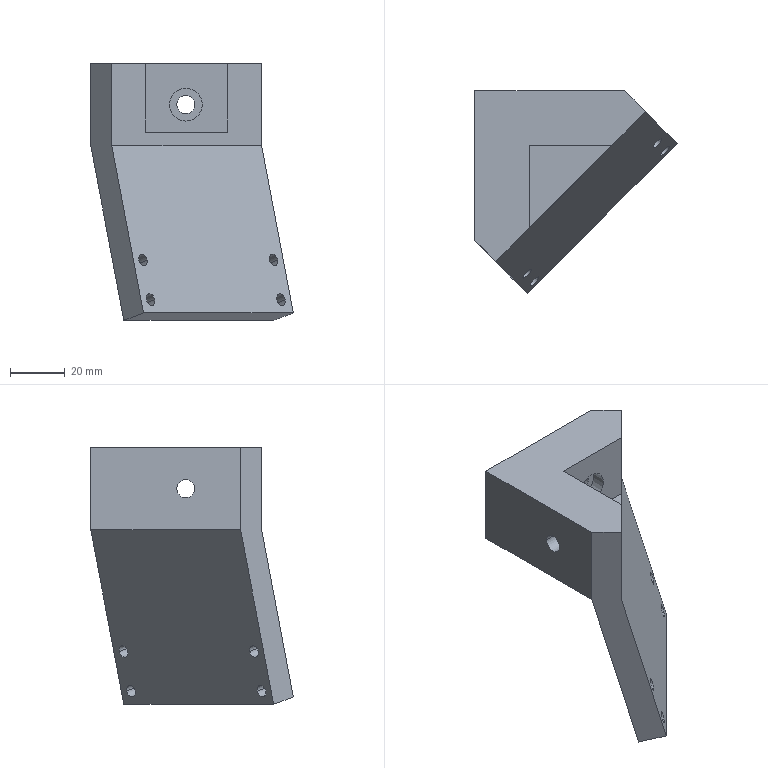Part | SolidWorks | features ICE 6, Extrusion 1, MirrorPattern 1 | 1 solid | 31 faces | box 73.918 x 73.918 x 93.747 mm | volume 108156 mm3 | cylinder 16 | plane 15 | commonest cylinder face diameters 4.4 x8 6.6 x4 12 x4
STEP:
#1=CARTESIAN_POINT('',(10.398,-61.143,-59.429));
#2=VERTEX_POINT('',#1);
#3=CARTESIAN_POINT('',(13.509,-58.031,-59.429));
#4=VERTEX_POINT('',#3);
#5=CARTESIAN_POINT('',(11.953,-59.587,-59.429));
#6=DIRECTION('',(0.683,-0.683,0.2588));
#7=DIRECTION('',(0.7071,0.7071,0.));
#8=AXIS2_PLACEMENT_3D('',#5,#6,#7);
#9=CIRCLE('',#8,2.2);
#10=EDGE_CURVE('',#2,#4,#9,.T.);
#11=ORIENTED_EDGE('',*,*,#10,.F.);
#12=CARTESIAN_POINT('',(17.533,-68.278,-56.725));
#13=VERTEX_POINT('',#12);
#14=CARTESIAN_POINT('',(-2.957,-47.788,-64.49));
#15=DIRECTION('',(0.683,-0.683,0.2588));
#16=VECTOR('',#15,1000.);
#17=LINE('',#14,#16);
#18=EDGE_CURVE('',#2,#13,#17,.T.);
#19=ORIENTED_EDGE('',*,*,#18,.T.);
#20=CARTESIAN_POINT('',(20.644,-65.167,-56.725));
#21=VERTEX_POINT('',#20);
#22=CARTESIAN_POINT('',(19.089,-66.722,-56.725));
#23=DIRECTION('',(0.683,-0.683,0.2588));
#24=DIRECTION('',(0.7071,0.7071,0.));
#25=AXIS2_PLACEMENT_3D('',#22,#23,#24);
#26=CIRCLE('',#25,2.2);
#27=EDGE_CURVE('',#13,#21,#26,.T.);
#28=ORIENTED_EDGE('',*,*,#27,.T.);
#29=CARTESIAN_POINT('',(0.1541,-44.676,-64.49));
#30=DIRECTION('',(0.683,-0.683,0.2588));
#31=VECTOR('',#30,1000.);
#32=LINE('',#29,#31);
#33=EDGE_CURVE('',#4,#21,#32,.T.);
#34=ORIENTED_EDGE('',*,*,#33,.F.);
#35=EDGE_LOOP('',(#11,#19,#28,#34));
#36=FACE_OUTER_BOUND('',#35,.T.);
#37=CARTESIAN_POINT('',(-1.402,-46.232,-64.49));
#38=DIRECTION('',(0.683,-0.683,0.2588));
#39=DIRECTION('',(0.7071,0.7071,0.));
#40=AXIS2_PLACEMENT_3D('',#37,#38,#39);
#41=CYLINDRICAL_SURFACE('',#40,2.2);
#42=ADVANCED_FACE('',(#36),#41,.F.);
#43=CARTESIAN_POINT('',(13.143,-63.888,-73.918));
#44=VERTEX_POINT('',#43);
#45=CARTESIAN_POINT('',(16.254,-60.776,-73.918));
#46=VERTEX_POINT('',#45);
#47=CARTESIAN_POINT('',(14.699,-62.332,-73.918));
#48=DIRECTION('',(0.683,-0.683,0.2588));
#49=DIRECTION('',(0.7071,0.7071,0.));
#50=AXIS2_PLACEMENT_3D('',#47,#48,#49);
#51=CIRCLE('',#50,2.2);
#52=EDGE_CURVE('',#44,#46,#51,.T.);
#53=ORIENTED_EDGE('',*,*,#52,.F.);
#54=CARTESIAN_POINT('',(20.278,-71.023,-71.214));
#55=VERTEX_POINT('',#54);
#56=CARTESIAN_POINT('',(-0.212,-50.533,-78.978));
#57=DIRECTION('',(0.683,-0.683,0.2588));
#58=VECTOR('',#57,1000.);
#59=LINE('',#56,#58);
#60=EDGE_CURVE('',#44,#55,#59,.T.);
#61=ORIENTED_EDGE('',*,*,#60,.T.);
#62=CARTESIAN_POINT('',(23.39,-67.912,-71.214));
#63=VERTEX_POINT('',#62);
#64=CARTESIAN_POINT('',(21.834,-69.468,-71.214));
#65=DIRECTION('',(0.683,-0.683,0.2588));
#66=DIRECTION('',(0.7071,0.7071,0.));
#67=AXIS2_PLACEMENT_3D('',#64,#65,#66);
#68=CIRCLE('',#67,2.2);
#69=EDGE_CURVE('',#55,#63,#68,.T.);
#70=ORIENTED_EDGE('',*,*,#69,.T.);
#71=CARTESIAN_POINT('',(2.899,-47.422,-78.978));
#72=DIRECTION('',(0.683,-0.683,0.2588));
#73=VECTOR('',#72,1000.);
#74=LINE('',#71,#73);
#75=EDGE_CURVE('',#46,#63,#74,.T.);
#76=ORIENTED_EDGE('',*,*,#75,.F.);
#77=EDGE_LOOP('',(#53,#61,#70,#76));
#78=FACE_OUTER_BOUND('',#77,.T.);
#79=CARTESIAN_POINT('',(1.344,-48.977,-78.978));
#80=DIRECTION('',(0.683,-0.683,0.2588));
#81=DIRECTION('',(0.7071,0.7071,0.));
#82=AXIS2_PLACEMENT_3D('',#79,#80,#81);
#83=CYLINDRICAL_SURFACE('',#82,2.2);
#84=ADVANCED_FACE('',(#78),#83,.F.);
#85=CARTESIAN_POINT('',(60.776,-16.254,-73.918));
#86=VERTEX_POINT('',#85);
#87=CARTESIAN_POINT('',(63.888,-13.143,-73.918));
#88=VERTEX_POINT('',#87);
#89=CARTESIAN_POINT('',(62.332,-14.699,-73.918));
#90=DIRECTION('',(0.683,-0.683,0.2588));
#91=DIRECTION('',(0.7071,0.7071,0.));
#92=AXIS2_PLACEMENT_3D('',#89,#90,#91);
#93=CIRCLE('',#92,2.2);
#94=EDGE_CURVE('',#86,#88,#93,.T.);
#95=ORIENTED_EDGE('',*,*,#94,.F.);
#96=CARTESIAN_POINT('',(67.912,-23.39,-71.214));
#97=VERTEX_POINT('',#96);
#98=CARTESIAN_POINT('',(47.422,-2.899,-78.978));
#99=DIRECTION('',(0.683,-0.683,0.2588));
#100=VECTOR('',#99,1000.);
#101=LINE('',#98,#100);
#102=EDGE_CURVE('',#86,#97,#101,.T.);
#103=ORIENTED_EDGE('',*,*,#102,.T.);
#104=CARTESIAN_POINT('',(71.023,-20.278,-71.214));
#105=VERTEX_POINT('',#104);
#106=CARTESIAN_POINT('',(69.468,-21.834,-71.214));
#107=DIRECTION('',(0.683,-0.683,0.2588));
#108=DIRECTION('',(0.7071,0.7071,0.));
#109=AXIS2_PLACEMENT_3D('',#106,#107,#108);
#110=CIRCLE('',#109,2.2);
#111=EDGE_CURVE('',#97,#105,#110,.T.);
#112=ORIENTED_EDGE('',*,*,#111,.T.);
#113=CARTESIAN_POINT('',(50.533,0.212,-78.978));
#114=DIRECTION('',(0.683,-0.683,0.2588));
#115=VECTOR('',#114,1000.);
#116=LINE('',#113,#115);
#117=EDGE_CURVE('',#88,#105,#116,.T.);
#118=ORIENTED_EDGE('',*,*,#117,.F.);
#119=EDGE_LOOP('',(#95,#103,#112,#118));
#120=FACE_OUTER_BOUND('',#119,.T.);
#121=CARTESIAN_POINT('',(48.977,-1.344,-78.978));
#122=DIRECTION('',(0.683,-0.683,0.2588));
#123=DIRECTION('',(0.7071,0.7071,0.));
#124=AXIS2_PLACEMENT_3D('',#121,#122,#123);
#125=CYLINDRICAL_SURFACE('',#124,2.2);
#126=ADVANCED_FACE('',(#120),#125,.F.);
#127=CARTESIAN_POINT('',(58.031,-13.509,-59.429));
#128=VERTEX_POINT('',#127);
#129=CARTESIAN_POINT('',(61.143,-10.398,-59.429));
#130=VERTEX_POINT('',#129);
#131=CARTESIAN_POINT('',(59.587,-11.953,-59.429));
#132=DIRECTION('',(0.683,-0.683,0.2588));
#133=DIRECTION('',(0.7071,0.7071,0.));
#134=AXIS2_PLACEMENT_3D('',#131,#132,#133);
#135=CIRCLE('',#134,2.2);
#136=EDGE_CURVE('',#128,#130,#135,.T.);
#137=ORIENTED_EDGE('',*,*,#136,.F.);
#138=CARTESIAN_POINT('',(65.167,-20.644,-56.725));
#139=VERTEX_POINT('',#138);
#140=CARTESIAN_POINT('',(44.676,-0.1541,-64.49));
#141=DIRECTION('',(0.683,-0.683,0.2588));
#142=VECTOR('',#141,1000.);
#143=LINE('',#140,#142);
#144=EDGE_CURVE('',#128,#139,#143,.T.);
#145=ORIENTED_EDGE('',*,*,#144,.T.);
#146=CARTESIAN_POINT('',(68.278,-17.533,-56.725));
#147=VERTEX_POINT('',#146);
#148=CARTESIAN_POINT('',(66.722,-19.089,-56.725));
#149=DIRECTION('',(0.683,-0.683,0.2588));
#150=DIRECTION('',(0.7071,0.7071,0.));
#151=AXIS2_PLACEMENT_3D('',#148,#149,#150);
#152=CIRCLE('',#151,2.2);
#153=EDGE_CURVE('',#139,#147,#152,.T.);
#154=ORIENTED_EDGE('',*,*,#153,.T.);
#155=CARTESIAN_POINT('',(47.788,2.957,-64.49));
#156=DIRECTION('',(0.683,-0.683,0.2588));
#157=VECTOR('',#156,1000.);
#158=LINE('',#155,#157);
#159=EDGE_CURVE('',#130,#147,#158,.T.);
#160=ORIENTED_EDGE('',*,*,#159,.F.);
#161=EDGE_LOOP('',(#137,#145,#154,#160));
#162=FACE_OUTER_BOUND('',#161,.T.);
#163=CARTESIAN_POINT('',(46.232,1.402,-64.49));
#164=DIRECTION('',(0.683,-0.683,0.2588));
#165=DIRECTION('',(0.7071,0.7071,0.));
#166=AXIS2_PLACEMENT_3D('',#163,#164,#165);
#167=CYLINDRICAL_SURFACE('',#166,2.2);
#168=ADVANCED_FACE('',(#162),#167,.F.);
#169=CARTESIAN_POINT('',(20.,-40.705,0.));
#170=VERTEX_POINT('',#169);
#171=CARTESIAN_POINT('',(20.,-28.705,0.));
#172=VERTEX_POINT('',#171);
#173=CARTESIAN_POINT('',(20.,-34.705,0.));
#174=DIRECTION('',(1.,0.,0.));
#175=DIRECTION('',(0.,-1.,0.));
#176=AXIS2_PLACEMENT_3D('',#173,#174,#175);
#177=CIRCLE('',#176,6.);
#178=EDGE_CURVE('',#170,#172,#177,.T.);
#179=ORIENTED_EDGE('',*,*,#178,.T.);
#180=CARTESIAN_POINT('',(15.,-28.705,0.));
#181=VERTEX_POINT('',#180);
#182=CARTESIAN_POINT('',(128.,-28.705,0.));
#183=DIRECTION('',(-1.,0.,0.));
#184=VECTOR('',#183,1000.);
#185=LINE('',#182,#184);
#186=EDGE_CURVE('',#172,#181,#185,.T.);
#187=ORIENTED_EDGE('',*,*,#186,.T.);
#188=CARTESIAN_POINT('',(15.,-40.705,0.));
#189=VERTEX_POINT('',#188);
#190=CARTESIAN_POINT('',(15.,-34.705,0.));
#191=DIRECTION('',(1.,0.,0.));
#192=DIRECTION('',(0.,0.,1.));
#193=AXIS2_PLACEMENT_3D('',#190,#191,#192);
#194=CIRCLE('',#193,6.);
#195=EDGE_CURVE('',#189,#181,#194,.T.);
#196=ORIENTED_EDGE('',*,*,#195,.F.);
#197=CARTESIAN_POINT('',(128.,-40.705,0.));
#198=DIRECTION('',(-1.,0.,0.));
#199=VECTOR('',#198,1000.);
#200=LINE('',#197,#199);
#201=EDGE_CURVE('',#170,#189,#200,.T.);
#202=ORIENTED_EDGE('',*,*,#201,.F.);
#203=EDGE_LOOP('',(#179,#187,#196,#202));
#204=FACE_OUTER_BOUND('',#203,.T.);
#205=CARTESIAN_POINT('',(128.,-34.705,0.));
#206=DIRECTION('',(-1.,0.,0.));
#207=DIRECTION('',(0.,-1.,0.));
#208=AXIS2_PLACEMENT_3D('',#205,#206,#207);
#209=CYLINDRICAL_SURFACE('',#208,6.);
#210=ADVANCED_FACE('',(#204),#209,.F.);
#211=CARTESIAN_POINT('',(15.,-31.405,0.));
#212=VERTEX_POINT('',#211);
#213=CARTESIAN_POINT('',(15.,-38.005,0.));
#214=VERTEX_POINT('',#213);
#215=CARTESIAN_POINT('',(15.,-34.705,0.));
#216=DIRECTION('',(-1.,0.,0.));
#217=DIRECTION('',(0.,-1.,0.));
#218=AXIS2_PLACEMENT_3D('',#215,#216,#217);
#219=CIRCLE('',#218,3.3);
#220=EDGE_CURVE('',#212,#214,#219,.T.);
#221=ORIENTED_EDGE('',*,*,#220,.F.);
#222=CARTESIAN_POINT('',(0.,-31.405,0.));
#223=VERTEX_POINT('',#222);
#224=CARTESIAN_POINT('',(113.,-31.405,0.));
#225=DIRECTION('',(-1.,0.,0.));
#226=VECTOR('',#225,1000.);
#227=LINE('',#224,#226);
#228=EDGE_CURVE('',#212,#223,#227,.T.);
#229=ORIENTED_EDGE('',*,*,#228,.T.);
#230=CARTESIAN_POINT('',(0.,-38.005,0.));
#231=VERTEX_POINT('',#230);
#232=CARTESIAN_POINT('',(0.,-34.705,0.));
#233=DIRECTION('',(1.,0.,0.));
#234=DIRECTION('',(0.,0.,1.));
#235=AXIS2_PLACEMENT_3D('',#232,#233,#234);
#236=CIRCLE('',#235,3.3);
#237=EDGE_CURVE('',#231,#223,#236,.T.);
#238=ORIENTED_EDGE('',*,*,#237,.F.);
#239=CARTESIAN_POINT('',(113.,-38.005,0.));
#240=DIRECTION('',(-1.,0.,0.));
#241=VECTOR('',#240,1000.);
#242=LINE('',#239,#241);
#243=EDGE_CURVE('',#214,#231,#242,.T.);
#244=ORIENTED_EDGE('',*,*,#243,.F.);
#245=EDGE_LOOP('',(#221,#229,#238,#244));
#246=FACE_OUTER_BOUND('',#245,.T.);
#247=CARTESIAN_POINT('',(113.,-34.705,0.));
#248=DIRECTION('',(-1.,0.,0.));
#249=DIRECTION('',(0.,-1.,0.));
#250=AXIS2_PLACEMENT_3D('',#247,#248,#249);
#251=CYLINDRICAL_SURFACE('',#250,3.3);
#252=ADVANCED_FACE('',(#246),#251,.F.);
#253=CARTESIAN_POINT('',(34.705,-20.,6.));
#254=VERTEX_POINT('',#253);
#255=CARTESIAN_POINT('',(34.705,-20.,-6.));
#256=VERTEX_POINT('',#255);
#257=CARTESIAN_POINT('',(34.705,-20.,0.));
#258=DIRECTION('',(0.,-1.,0.));
#259=DIRECTION('',(0.,0.,1.));
#260=AXIS2_PLACEMENT_3D('',#257,#258,#259);
#261=CIRCLE('',#260,6.);
#262=EDGE_CURVE('',#254,#256,#261,.T.);
#263=ORIENTED_EDGE('',*,*,#262,.T.);
#264=CARTESIAN_POINT('',(34.705,-15.,-6.));
#265=VERTEX_POINT('',#264);
#266=CARTESIAN_POINT('',(34.705,-128.,-6.));
#267=DIRECTION('',(0.,1.,0.));
#268=VECTOR('',#267,1000.);
#269=LINE('',#266,#268);
#270=EDGE_CURVE('',#256,#265,#269,.T.);
#271=ORIENTED_EDGE('',*,*,#270,.T.);
#272=CARTESIAN_POINT('',(34.705,-15.,6.));
#273=VERTEX_POINT('',#272);
#274=CARTESIAN_POINT('',(34.705,-15.,0.));
#275=DIRECTION('',(0.,1.,0.));
#276=DIRECTION('',(0.,0.,1.));
#277=AXIS2_PLACEMENT_3D('',#274,#275,#276);
#278=CIRCLE('',#277,6.);
#279=EDGE_CURVE('',#265,#273,#278,.T.);
#280=ORIENTED_EDGE('',*,*,#279,.T.);
#281=CARTESIAN_POINT('',(34.705,-128.,6.));
#282=DIRECTION('',(0.,1.,0.));
#283=VECTOR('',#282,1000.);
#284=LINE('',#281,#283);
#285=EDGE_CURVE('',#254,#273,#284,.T.);
#286=ORIENTED_EDGE('',*,*,#285,.F.);
#287=EDGE_LOOP('',(#263,#271,#280,#286));
#288=FACE_OUTER_BOUND('',#287,.T.);
#289=CARTESIAN_POINT('',(34.705,-128.,0.));
#290=DIRECTION('',(0.,1.,0.));
#291=DIRECTION('',(0.,0.,1.));
#292=AXIS2_PLACEMENT_3D('',#289,#290,#291);
#293=CYLINDRICAL_SURFACE('',#292,6.);
#294=ADVANCED_FACE('',(#288),#293,.F.);
#295=CARTESIAN_POINT('',(34.705,-15.,3.3));
#296=VERTEX_POINT('',#295);
#297=CARTESIAN_POINT('',(34.705,-15.,-3.3));
#298=VERTEX_POINT('',#297);
#299=CARTESIAN_POINT('',(34.705,-15.,0.));
#300=DIRECTION('',(0.,-1.,0.));
#301=DIRECTION('',(0.,0.,1.));
#302=AXIS2_PLACEMENT_3D('',#299,#300,#301);
#303=CIRCLE('',#302,3.3);
#304=EDGE_CURVE('',#296,#298,#303,.T.);
#305=ORIENTED_EDGE('',*,*,#304,.T.);
#306=CARTESIAN_POINT('',(34.705,0.,-3.3));
#307=VERTEX_POINT('',#306);
#308=CARTESIAN_POINT('',(34.705,-113.,-3.3));
#309=DIRECTION('',(0.,1.,0.));
#310=VECTOR('',#309,1000.);
#311=LINE('',#308,#310);
#312=EDGE_CURVE('',#298,#307,#311,.T.);
#313=ORIENTED_EDGE('',*,*,#312,.T.);
#314=CARTESIAN_POINT('',(34.705,0.,3.3));
#315=VERTEX_POINT('',#314);
#316=CARTESIAN_POINT('',(34.705,0.,0.));
#317=DIRECTION('',(0.,1.,0.));
#318=DIRECTION('',(0.,0.,1.));
#319=AXIS2_PLACEMENT_3D('',#316,#317,#318);
#320=CIRCLE('',#319,3.3);
#321=EDGE_CURVE('',#307,#315,#320,.T.);
#322=ORIENTED_EDGE('',*,*,#321,.T.);
#323=CARTESIAN_POINT('',(34.705,-113.,3.3));
#324=DIRECTION('',(0.,1.,0.));
#325=VECTOR('',#324,1000.);
#326=LINE('',#323,#325);
#327=EDGE_CURVE('',#296,#315,#326,.T.);
#328=ORIENTED_EDGE('',*,*,#327,.F.);
#329=EDGE_LOOP('',(#305,#313,#322,#328));
#330=FACE_OUTER_BOUND('',#329,.T.);
#331=CARTESIAN_POINT('',(34.705,-113.,0.));
#332=DIRECTION('',(0.,1.,0.));
#333=DIRECTION('',(0.,0.,1.));
#334=AXIS2_PLACEMENT_3D('',#331,#332,#333);
#335=CYLINDRICAL_SURFACE('',#334,3.3);
#336=ADVANCED_FACE('',(#330),#335,.F.);
#337=CARTESIAN_POINT('',(20.,-50.,-10.));
#338=VERTEX_POINT('',#337);
#339=CARTESIAN_POINT('',(50.,-20.,-10.));
#340=VERTEX_POINT('',#339);
#341=CARTESIAN_POINT('',(35.,-35.,-10.));
#342=DIRECTION('',(0.7071,0.7071,0.));
#343=VECTOR('',#342,1000.);
#344=LINE('',#341,#343);
#345=EDGE_CURVE('',#338,#340,#344,.T.);
#346=ORIENTED_EDGE('',*,*,#345,.F.);
#347=CARTESIAN_POINT('',(20.,-50.,15.));
#348=VERTEX_POINT('',#347);
#349=CARTESIAN_POINT('',(20.,-50.,-10.));
#350=DIRECTION('',(0.,0.,1.));
#351=VECTOR('',#350,1000.);
#352=LINE('',#349,#351);
#353=EDGE_CURVE('',#338,#348,#352,.T.);
#354=ORIENTED_EDGE('',*,*,#353,.T.);
#355=CARTESIAN_POINT('',(7.648,-62.352,15.));
#356=VERTEX_POINT('',#355);
#357=CARTESIAN_POINT('',(70.,0.,15.));
#358=DIRECTION('',(0.7071,0.7071,0.));
#359=VECTOR('',#358,1000.);
#360=LINE('',#357,#359);
#361=EDGE_CURVE('',#356,#348,#360,.T.);
#362=ORIENTED_EDGE('',*,*,#361,.F.);
#363=CARTESIAN_POINT('',(7.648,-62.352,-15.));
#364=VERTEX_POINT('',#363);
#365=CARTESIAN_POINT('',(7.648,-62.352,15.));
#366=DIRECTION('',(0.,0.,1.));
#367=VECTOR('',#366,1000.);
#368=LINE('',#365,#367);
#369=EDGE_CURVE('',#364,#356,#368,.T.);
#370=ORIENTED_EDGE('',*,*,#369,.F.);
#371=CARTESIAN_POINT('',(62.352,-7.648,-15.));
#372=VERTEX_POINT('',#371);
#373=CARTESIAN_POINT('',(70.,0.,-15.));
#374=DIRECTION('',(0.7071,0.7071,0.));
#375=VECTOR('',#374,1000.);
#376=LINE('',#373,#375);
#377=EDGE_CURVE('',#364,#372,#376,.T.);
#378=ORIENTED_EDGE('',*,*,#377,.T.);
#379=CARTESIAN_POINT('',(62.352,-7.648,15.));
#380=VERTEX_POINT('',#379);
#381=CARTESIAN_POINT('',(62.352,-7.648,15.));
#382=DIRECTION('',(0.,0.,1.));
#383=VECTOR('',#382,1000.);
#384=LINE('',#381,#383);
#385=EDGE_CURVE('',#372,#380,#384,.T.);
#386=ORIENTED_EDGE('',*,*,#385,.T.);
#387=CARTESIAN_POINT('',(50.,-20.,15.));
#388=VERTEX_POINT('',#387);
#389=CARTESIAN_POINT('',(70.,0.,15.));
#390=DIRECTION('',(0.7071,0.7071,0.));
#391=VECTOR('',#390,1000.);
#392=LINE('',#389,#391);
#393=EDGE_CURVE('',#388,#380,#392,.T.);
#394=ORIENTED_EDGE('',*,*,#393,.F.);
#395=CARTESIAN_POINT('',(50.,-20.,-10.));
#396=DIRECTION('',(0.,0.,1.));
#397=VECTOR('',#396,1000.);
#398=LINE('',#395,#397);
#399=EDGE_CURVE('',#340,#388,#398,.T.);
#400=ORIENTED_EDGE('',*,*,#399,.F.);
#401=EDGE_LOOP('',(#346,#354,#362,#370,#378,#386,#394,#400));
#402=FACE_OUTER_BOUND('',#401,.T.);
#403=CARTESIAN_POINT('',(70.,0.,15.));
#404=DIRECTION('',(-0.7071,0.7071,0.));
#405=DIRECTION('',(-0.7071,-0.7071,0.));
#406=AXIS2_PLACEMENT_3D('',#403,#404,#405);
#407=PLANE('',#406);
#408=ADVANCED_FACE('',(#402),#407,.F.);
#409=ORIENTED_EDGE('',*,*,#361,.T.);
#410=CARTESIAN_POINT('',(20.,-20.,15.));
#411=VERTEX_POINT('',#410);
#412=CARTESIAN_POINT('',(20.,0.,15.));
#413=DIRECTION('',(0.,-1.,0.));
#414=VECTOR('',#413,1000.);
#415=LINE('',#412,#414);
#416=EDGE_CURVE('',#411,#348,#415,.T.);
#417=ORIENTED_EDGE('',*,*,#416,.F.);
#418=CARTESIAN_POINT('',(0.,-20.,15.));
#419=DIRECTION('',(-1.,0.,0.));
#420=VECTOR('',#419,1000.);
#421=LINE('',#418,#420);
#422=EDGE_CURVE('',#388,#411,#421,.T.);
#423=ORIENTED_EDGE('',*,*,#422,.F.);
#424=ORIENTED_EDGE('',*,*,#393,.T.);
#425=CARTESIAN_POINT('',(54.705,0.,15.));
#426=VERTEX_POINT('',#425);
#427=CARTESIAN_POINT('',(27.352,27.352,15.));
#428=DIRECTION('',(0.7071,-0.7071,0.));
#429=VECTOR('',#428,1000.);
#430=LINE('',#427,#429);
#431=EDGE_CURVE('',#426,#380,#430,.T.);
#432=ORIENTED_EDGE('',*,*,#431,.F.);
#433=CARTESIAN_POINT('',(0.,0.,15.));
#434=VERTEX_POINT('',#433);
#435=CARTESIAN_POINT('',(0.,0.,15.));
#436=DIRECTION('',(-1.,0.,0.));
#437=VECTOR('',#436,1000.);
#438=LINE('',#435,#437);
#439=EDGE_CURVE('',#426,#434,#438,.T.);
#440=ORIENTED_EDGE('',*,*,#439,.T.);
#441=CARTESIAN_POINT('',(0.,-54.705,15.));
#442=VERTEX_POINT('',#441);
#443=CARTESIAN_POINT('',(0.,-70.,15.));
#444=DIRECTION('',(0.,-1.,0.));
#445=VECTOR('',#444,1000.);
#446=LINE('',#443,#445);
#447=EDGE_CURVE('',#434,#442,#446,.T.);
#448=ORIENTED_EDGE('',*,*,#447,.T.);
#449=CARTESIAN_POINT('',(-27.352,-27.352,15.));
#450=DIRECTION('',(0.7071,-0.7071,0.));
#451=VECTOR('',#450,1000.);
#452=LINE('',#449,#451);
#453=EDGE_CURVE('',#442,#356,#452,.T.);
#454=ORIENTED_EDGE('',*,*,#453,.T.);
#455=EDGE_LOOP('',(#409,#417,#423,#424,#432,#440,#448,#454));
#456=FACE_OUTER_BOUND('',#455,.T.);
#457=CARTESIAN_POINT('',(0.,0.,15.));
#458=DIRECTION('',(0.,0.,-1.));
#459=DIRECTION('',(-1.,0.,0.));
#460=AXIS2_PLACEMENT_3D('',#457,#458,#459);
#461=PLANE('',#460);
#462=ADVANCED_FACE('',(#456),#461,.F.);
#463=CARTESIAN_POINT('',(11.953,-59.587,-59.429));
#464=DIRECTION('',(0.683,-0.683,0.2588));
#465=DIRECTION('',(0.7071,0.7071,0.));
#466=AXIS2_PLACEMENT_3D('',#463,#464,#465);
#467=CIRCLE('',#466,2.2);
#468=EDGE_CURVE('',#4,#2,#467,.T.);
#469=ORIENTED_EDGE('',*,*,#468,.T.);
#470=ORIENTED_EDGE('',*,*,#10,.T.);
#471=EDGE_LOOP('',(#469,#470));
#472=FACE_BOUND('',#471,.T.);
#473=CARTESIAN_POINT('',(14.699,-62.332,-73.918));
#474=DIRECTION('',(0.683,-0.683,0.2588));
#475=DIRECTION('',(0.7071,0.7071,0.));
#476=AXIS2_PLACEMENT_3D('',#473,#474,#475);
#477=CIRCLE('',#476,2.2);
#478=EDGE_CURVE('',#46,#44,#477,.T.);
#479=ORIENTED_EDGE('',*,*,#478,.T.);
#480=ORIENTED_EDGE('',*,*,#52,.T.);
#481=EDGE_LOOP('',(#479,#480));
#482=FACE_BOUND('',#481,.T.);
#483=CARTESIAN_POINT('',(62.332,-14.699,-73.918));
#484=DIRECTION('',(0.683,-0.683,0.2588));
#485=DIRECTION('',(0.7071,0.7071,0.));
#486=AXIS2_PLACEMENT_3D('',#483,#484,#485);
#487=CIRCLE('',#486,2.2);
#488=EDGE_CURVE('',#88,#86,#487,.T.);
#489=ORIENTED_EDGE('',*,*,#488,.T.);
#490=ORIENTED_EDGE('',*,*,#94,.T.);
#491=EDGE_LOOP('',(#489,#490));
#492=FACE_BOUND('',#491,.T.);
#493=CARTESIAN_POINT('',(59.587,-11.953,-59.429));
#494=DIRECTION('',(0.683,-0.683,0.2588));
#495=DIRECTION('',(0.7071,0.7071,0.));
#496=AXIS2_PLACEMENT_3D('',#493,#494,#495);
#497=CIRCLE('',#496,2.2);
#498=EDGE_CURVE('',#130,#128,#497,.T.);
#499=ORIENTED_EDGE('',*,*,#498,.T.);
#500=ORIENTED_EDGE('',*,*,#136,.T.);
#501=EDGE_LOOP('',(#499,#500));
#502=FACE_BOUND('',#501,.T.);
#503=CARTESIAN_POINT('',(0.,-54.705,-15.));
#504=VERTEX_POINT('',#503);
#505=CARTESIAN_POINT('',(54.705,0.,-15.));
#506=VERTEX_POINT('',#505);
#507=CARTESIAN_POINT('',(-7.648,-62.352,-15.));
#508=DIRECTION('',(0.7071,0.7071,0.));
#509=VECTOR('',#508,1000.);
#510=LINE('',#507,#509);
#511=EDGE_CURVE('',#504,#506,#510,.T.);
#512=ORIENTED_EDGE('',*,*,#511,.T.);
#513=CARTESIAN_POINT('',(66.783,-12.078,-78.747));
#514=VERTEX_POINT('',#513);
#515=CARTESIAN_POINT('',(50.221,4.484,8.666));
#516=DIRECTION('',(0.183,-0.183,-0.9659));
#517=VECTOR('',#516,1000.);
#518=LINE('',#515,#517);
#519=EDGE_CURVE('',#506,#514,#518,.T.);
#520=ORIENTED_EDGE('',*,*,#519,.T.);
#521=CARTESIAN_POINT('',(12.078,-66.783,-78.747));
#522=VERTEX_POINT('',#521);
#523=CARTESIAN_POINT('',(4.43,-74.43,-78.747));
#524=DIRECTION('',(0.7071,0.7071,0.));
#525=VECTOR('',#524,1000.);
#526=LINE('',#523,#525);
#527=EDGE_CURVE('',#522,#514,#526,.T.);
#528=ORIENTED_EDGE('',*,*,#527,.F.);
#529=CARTESIAN_POINT('',(-4.484,-50.221,8.666));
#530=DIRECTION('',(0.183,-0.183,-0.9659));
#531=VECTOR('',#530,1000.);
#532=LINE('',#529,#531);
#533=EDGE_CURVE('',#504,#522,#532,.T.);
#534=ORIENTED_EDGE('',*,*,#533,.F.);
#535=EDGE_LOOP('',(#512,#520,#528,#534));
#536=FACE_OUTER_BOUND('',#535,.T.);
#537=CARTESIAN_POINT('',(-12.132,-57.868,8.666));
#538=DIRECTION('',(0.683,-0.683,0.2588));
#539=DIRECTION('',(0.7071,0.7071,0.));
#540=AXIS2_PLACEMENT_3D('',#537,#538,#539);
#541=PLANE('',#540);
#542=ADVANCED_FACE('',(#472,#482,#492,#502,#536),#541,.F.);
#543=ORIENTED_EDGE('',*,*,#527,.T.);
#544=CARTESIAN_POINT('',(73.918,-19.214,-76.044));
#545=VERTEX_POINT('',#544);
#546=CARTESIAN_POINT('',(43.914,10.79,-87.413));
#547=DIRECTION('',(0.683,-0.683,0.2588));
#548=VECTOR('',#547,1000.);
#549=LINE('',#546,#548);
#550=EDGE_CURVE('',#514,#545,#549,.T.);
#551=ORIENTED_EDGE('',*,*,#550,.T.);
#552=CARTESIAN_POINT('',(19.214,-73.918,-76.044));
#553=VERTEX_POINT('',#552);
#554=CARTESIAN_POINT('',(11.566,-81.566,-76.044));
#555=DIRECTION('',(0.7071,0.7071,0.));
#556=VECTOR('',#555,1000.);
#557=LINE('',#554,#556);
#558=EDGE_CURVE('',#553,#545,#557,.T.);
#559=ORIENTED_EDGE('',*,*,#558,.F.);
#560=CARTESIAN_POINT('',(-10.79,-43.914,-87.413));
#561=DIRECTION('',(0.683,-0.683,0.2588));
#562=VECTOR('',#561,1000.);
#563=LINE('',#560,#562);
#564=EDGE_CURVE('',#522,#553,#563,.T.);
#565=ORIENTED_EDGE('',*,*,#564,.F.);
#566=EDGE_LOOP('',(#543,#551,#559,#565));
#567=FACE_OUTER_BOUND('',#566,.T.);
#568=CARTESIAN_POINT('',(-18.438,-51.562,-87.413));
#569=DIRECTION('',(-0.183,0.183,0.9659));
#570=DIRECTION('',(0.9825,0.,0.1862));
#571=AXIS2_PLACEMENT_3D('',#568,#569,#570);
#572=PLANE('',#571);
#573=ADVANCED_FACE('',(#567),#572,.F.);
#574=CARTESIAN_POINT('',(19.089,-66.722,-56.725));
#575=DIRECTION('',(0.683,-0.683,0.2588));
#576=DIRECTION('',(0.7071,0.7071,0.));
#577=AXIS2_PLACEMENT_3D('',#574,#575,#576);
#578=CIRCLE('',#577,2.2);
#579=EDGE_CURVE('',#21,#13,#578,.T.);
#580=ORIENTED_EDGE('',*,*,#579,.F.);
#581=ORIENTED_EDGE('',*,*,#27,.F.);
#582=EDGE_LOOP('',(#580,#581));
#583=FACE_BOUND('',#582,.T.);
#584=CARTESIAN_POINT('',(21.834,-69.468,-71.214));
#585=DIRECTION('',(0.683,-0.683,0.2588));
#586=DIRECTION('',(0.7071,0.7071,0.));
#587=AXIS2_PLACEMENT_3D('',#584,#585,#586);
#588=CIRCLE('',#587,2.2);
#589=EDGE_CURVE('',#63,#55,#588,.T.);
#590=ORIENTED_EDGE('',*,*,#589,.F.);
#591=ORIENTED_EDGE('',*,*,#69,.F.);
#592=EDGE_LOOP('',(#590,#591));
#593=FACE_BOUND('',#592,.T.);
#594=CARTESIAN_POINT('',(69.468,-21.834,-71.214));
#595=DIRECTION('',(0.683,-0.683,0.2588));
#596=DIRECTION('',(0.7071,0.7071,0.));
#597=AXIS2_PLACEMENT_3D('',#594,#595,#596);
#598=CIRCLE('',#597,2.2);
#599=EDGE_CURVE('',#105,#97,#598,.T.);
#600=ORIENTED_EDGE('',*,*,#599,.F.);
#601=ORIENTED_EDGE('',*,*,#111,.F.);
#602=EDGE_LOOP('',(#600,#601));
#603=FACE_BOUND('',#602,.T.);
#604=CARTESIAN_POINT('',(66.722,-19.089,-56.725));
#605=DIRECTION('',(0.683,-0.683,0.2588));
#606=DIRECTION('',(0.7071,0.7071,0.));
#607=AXIS2_PLACEMENT_3D('',#604,#605,#606);
#608=CIRCLE('',#607,2.2);
#609=EDGE_CURVE('',#147,#139,#608,.T.);
#610=ORIENTED_EDGE('',*,*,#609,.F.);
#611=ORIENTED_EDGE('',*,*,#153,.F.);
#612=EDGE_LOOP('',(#610,#611));
#613=FACE_BOUND('',#612,.T.);
#614=CARTESIAN_POINT('',(57.356,-2.652,11.37));
#615=DIRECTION('',(0.183,-0.183,-0.9659));
#616=VECTOR('',#615,1000.);
#617=LINE('',#614,#616);
#618=EDGE_CURVE('',#372,#545,#617,.T.);
#619=ORIENTED_EDGE('',*,*,#618,.F.);
#620=ORIENTED_EDGE('',*,*,#377,.F.);
#621=CARTESIAN_POINT('',(2.652,-57.356,11.37));
#622=DIRECTION('',(0.183,-0.183,-0.9659));
#623=VECTOR('',#622,1000.);
#624=LINE('',#621,#623);
#625=EDGE_CURVE('',#364,#553,#624,.T.);
#626=ORIENTED_EDGE('',*,*,#625,.T.);
#627=ORIENTED_EDGE('',*,*,#558,.T.);
#628=EDGE_LOOP('',(#619,#620,#626,#627));
#629=FACE_OUTER_BOUND('',#628,.T.);
#630=CARTESIAN_POINT('',(-4.996,-65.004,11.37));
#631=DIRECTION('',(0.683,-0.683,0.2588));
#632=DIRECTION('',(0.7071,0.7071,0.));
#633=AXIS2_PLACEMENT_3D('',#630,#631,#632);
#634=PLANE('',#633);
#635=ADVANCED_FACE('',(#583,#593,#603,#613,#629),#634,.T.);
#636=ORIENTED_EDGE('',*,*,#237,.T.);
#637=CARTESIAN_POINT('',(0.,-34.705,0.));
#638=DIRECTION('',(1.,0.,0.));
#639=DIRECTION('',(0.,0.,1.));
#640=AXIS2_PLACEMENT_3D('',#637,#638,#639);
#641=CIRCLE('',#640,3.3);
#642=EDGE_CURVE('',#223,#231,#641,.T.);
#643=ORIENTED_EDGE('',*,*,#642,.T.);
#644=EDGE_LOOP('',(#636,#643));
#645=FACE_BOUND('',#644,.T.);
#646=CARTESIAN_POINT('',(0.,0.,-15.));
#647=VERTEX_POINT('',#646);
#648=CARTESIAN_POINT('',(0.,-70.,-15.));
#649=DIRECTION('',(0.,-1.,0.));
#650=VECTOR('',#649,1000.);
#651=LINE('',#648,#650);
#652=EDGE_CURVE('',#647,#504,#651,.T.);
#653=ORIENTED_EDGE('',*,*,#652,.T.);
#654=CARTESIAN_POINT('',(0.,-54.705,-98.));
#655=DIRECTION('',(0.,0.,1.));
#656=VECTOR('',#655,1000.);
#657=LINE('',#654,#656);
#658=EDGE_CURVE('',#504,#442,#657,.T.);
#659=ORIENTED_EDGE('',*,*,#658,.T.);
#660=ORIENTED_EDGE('',*,*,#447,.F.);
#661=CARTESIAN_POINT('',(0.,0.,15.));
#662=DIRECTION('',(0.,0.,-1.));
#663=VECTOR('',#662,1000.);
#664=LINE('',#661,#663);
#665=EDGE_CURVE('',#434,#647,#664,.T.);
#666=ORIENTED_EDGE('',*,*,#665,.T.);
#667=EDGE_LOOP('',(#653,#659,#660,#666));
#668=FACE_OUTER_BOUND('',#667,.T.);
#669=CARTESIAN_POINT('',(0.,-70.,15.));
#670=DIRECTION('',(1.,0.,0.));
#671=DIRECTION('',(0.,0.,-1.));
#672=AXIS2_PLACEMENT_3D('',#669,#670,#671);
#673=PLANE('',#672);
#674=ADVANCED_FACE('',(#645,#668),#673,.F.);
#675=CARTESIAN_POINT('',(34.705,0.,0.));
#676=DIRECTION('',(0.,1.,0.));
#677=DIRECTION('',(0.,0.,1.));
#678=AXIS2_PLACEMENT_3D('',#675,#676,#677);
#679=CIRCLE('',#678,3.3);
#680=EDGE_CURVE('',#315,#307,#679,.T.);
#681=ORIENTED_EDGE('',*,*,#680,.F.);
#682=ORIENTED_EDGE('',*,*,#321,.F.);
#683=EDGE_LOOP('',(#681,#682));
#684=FACE_BOUND('',#683,.T.);
#685=ORIENTED_EDGE('',*,*,#439,.F.);
#686=CARTESIAN_POINT('',(54.705,0.,-98.));
#687=DIRECTION('',(0.,0.,1.));
#688=VECTOR('',#687,1000.);
#689=LINE('',#686,#688);
#690=EDGE_CURVE('',#506,#426,#689,.T.);
#691=ORIENTED_EDGE('',*,*,#690,.F.);
#692=CARTESIAN_POINT('',(0.,0.,-15.));
#693=DIRECTION('',(-1.,0.,0.));
#694=VECTOR('',#693,1000.);
#695=LINE('',#692,#694);
#696=EDGE_CURVE('',#506,#647,#695,.T.);
#697=ORIENTED_EDGE('',*,*,#696,.T.);
#698=ORIENTED_EDGE('',*,*,#665,.F.);
#699=EDGE_LOOP('',(#685,#691,#697,#698));
#700=FACE_OUTER_BOUND('',#699,.T.);
#701=CARTESIAN_POINT('',(0.,0.,15.));
#702=DIRECTION('',(0.,-1.,0.));
#703=DIRECTION('',(0.,0.,-1.));
#704=AXIS2_PLACEMENT_3D('',#701,#702,#703);
#705=PLANE('',#704);
#706=ADVANCED_FACE('',(#684,#700),#705,.F.);
#707=ORIENTED_EDGE('',*,*,#511,.F.);
#708=ORIENTED_EDGE('',*,*,#652,.F.);
#709=ORIENTED_EDGE('',*,*,#696,.F.);
#710=EDGE_LOOP('',(#707,#708,#709));
#711=FACE_OUTER_BOUND('',#710,.T.);
#712=CARTESIAN_POINT('',(0.,0.,-15.));
#713=DIRECTION('',(0.,0.,-1.));
#714=DIRECTION('',(-1.,0.,0.));
#715=AXIS2_PLACEMENT_3D('',#712,#713,#714);
#716=PLANE('',#715);
#717=ADVANCED_FACE('',(#711),#716,.T.);
#718=ORIENTED_EDGE('',*,*,#369,.T.);
#719=ORIENTED_EDGE('',*,*,#453,.F.);
#720=ORIENTED_EDGE('',*,*,#658,.F.);
#721=ORIENTED_EDGE('',*,*,#533,.T.);
#722=ORIENTED_EDGE('',*,*,#564,.T.);
#723=ORIENTED_EDGE('',*,*,#625,.F.);
#724=EDGE_LOOP('',(#718,#719,#720,#721,#722,#723));
#725=FACE_OUTER_BOUND('',#724,.T.);
#726=CARTESIAN_POINT('',(-27.352,-27.352,-98.));
#727=DIRECTION('',(-0.7071,-0.7071,0.));
#728=DIRECTION('',(0.7071,-0.7071,0.));
#729=AXIS2_PLACEMENT_3D('',#726,#727,#728);
#730=PLANE('',#729);
#731=ADVANCED_FACE('',(#725),#730,.T.);
#732=ORIENTED_EDGE('',*,*,#618,.T.);
#733=ORIENTED_EDGE('',*,*,#550,.F.);
#734=ORIENTED_EDGE('',*,*,#519,.F.);
#735=ORIENTED_EDGE('',*,*,#690,.T.);
#736=ORIENTED_EDGE('',*,*,#431,.T.);
#737=ORIENTED_EDGE('',*,*,#385,.F.);
#738=EDGE_LOOP('',(#732,#733,#734,#735,#736,#737));
#739=FACE_OUTER_BOUND('',#738,.T.);
#740=CARTESIAN_POINT('',(27.352,27.352,-98.));
#741=DIRECTION('',(-0.7071,-0.7071,0.));
#742=DIRECTION('',(0.7071,-0.7071,0.));
#743=AXIS2_PLACEMENT_3D('',#740,#741,#742);
#744=PLANE('',#743);
#745=ADVANCED_FACE('',(#739),#744,.F.);
#746=ORIENTED_EDGE('',*,*,#312,.F.);
#747=CARTESIAN_POINT('',(34.705,-15.,0.));
#748=DIRECTION('',(0.,-1.,0.));
#749=DIRECTION('',(0.,0.,1.));
#750=AXIS2_PLACEMENT_3D('',#747,#748,#749);
#751=CIRCLE('',#750,3.3);
#752=EDGE_CURVE('',#298,#296,#751,.T.);
#753=ORIENTED_EDGE('',*,*,#752,.T.);
#754=ORIENTED_EDGE('',*,*,#327,.T.);
#755=ORIENTED_EDGE('',*,*,#680,.T.);
#756=EDGE_LOOP('',(#746,#753,#754,#755));
#757=FACE_OUTER_BOUND('',#756,.T.);
#758=CARTESIAN_POINT('',(34.705,-113.,0.));
#759=DIRECTION('',(0.,1.,0.));
#760=DIRECTION('',(0.,0.,1.));
#761=AXIS2_PLACEMENT_3D('',#758,#759,#760);
#762=CYLINDRICAL_SURFACE('',#761,3.3);
#763=ADVANCED_FACE('',(#757),#762,.F.);
#764=ORIENTED_EDGE('',*,*,#270,.F.);
#765=CARTESIAN_POINT('',(34.705,-20.,0.));
#766=DIRECTION('',(0.,-1.,0.));
#767=DIRECTION('',(0.,0.,1.));
#768=AXIS2_PLACEMENT_3D('',#765,#766,#767);
#769=CIRCLE('',#768,6.);
#770=EDGE_CURVE('',#256,#254,#769,.T.);
#771=ORIENTED_EDGE('',*,*,#770,.T.);
#772=ORIENTED_EDGE('',*,*,#285,.T.);
#773=CARTESIAN_POINT('',(34.705,-15.,0.));
#774=DIRECTION('',(0.,1.,0.));
#775=DIRECTION('',(0.,0.,1.));
#776=AXIS2_PLACEMENT_3D('',#773,#774,#775);
#777=CIRCLE('',#776,6.);
#778=EDGE_CURVE('',#273,#265,#777,.T.);
#779=ORIENTED_EDGE('',*,*,#778,.T.);
#780=EDGE_LOOP('',(#764,#771,#772,#779));
#781=FACE_OUTER_BOUND('',#780,.T.);
#782=CARTESIAN_POINT('',(34.705,-128.,0.));
#783=DIRECTION('',(0.,1.,0.));
#784=DIRECTION('',(0.,0.,1.));
#785=AXIS2_PLACEMENT_3D('',#782,#783,#784);
#786=CYLINDRICAL_SURFACE('',#785,6.);
#787=ADVANCED_FACE('',(#781),#786,.F.);
#788=ORIENTED_EDGE('',*,*,#778,.F.);
#789=ORIENTED_EDGE('',*,*,#279,.F.);
#790=EDGE_LOOP('',(#788,#789));
#791=FACE_OUTER_BOUND('',#790,.T.);
#792=ORIENTED_EDGE('',*,*,#304,.F.);
#793=ORIENTED_EDGE('',*,*,#752,.F.);
#794=EDGE_LOOP('',(#792,#793));
#795=FACE_BOUND('',#794,.T.);
#796=CARTESIAN_POINT('',(34.705,-15.,0.));
#797=DIRECTION('',(0.,1.,0.));
#798=DIRECTION('',(0.,0.,1.));
#799=AXIS2_PLACEMENT_3D('',#796,#797,#798);
#800=PLANE('',#799);
#801=ADVANCED_FACE('',(#791,#795),#800,.F.);
#802=ORIENTED_EDGE('',*,*,#422,.T.);
#803=CARTESIAN_POINT('',(20.,-20.,-10.));
#804=VERTEX_POINT('',#803);
#805=CARTESIAN_POINT('',(20.,-20.,-10.));
#806=DIRECTION('',(0.,0.,1.));
#807=VECTOR('',#806,1000.);
#808=LINE('',#805,#807);
#809=EDGE_CURVE('',#804,#411,#808,.T.);
#810=ORIENTED_EDGE('',*,*,#809,.F.);
#811=CARTESIAN_POINT('',(0.,-20.,-10.));
#812=DIRECTION('',(-1.,0.,0.));
#813=VECTOR('',#812,1000.);
#814=LINE('',#811,#813);
#815=EDGE_CURVE('',#340,#804,#814,.T.);
#816=ORIENTED_EDGE('',*,*,#815,.F.);
#817=ORIENTED_EDGE('',*,*,#399,.T.);
#818=EDGE_LOOP('',(#802,#810,#816,#817));
#819=FACE_OUTER_BOUND('',#818,.T.);
#820=ORIENTED_EDGE('',*,*,#262,.F.);
#821=ORIENTED_EDGE('',*,*,#770,.F.);
#822=EDGE_LOOP('',(#820,#821));
#823=FACE_BOUND('',#822,.T.);
#824=CARTESIAN_POINT('',(0.,-20.,-10.));
#825=DIRECTION('',(0.,1.,0.));
#826=DIRECTION('',(0.,0.,1.));
#827=AXIS2_PLACEMENT_3D('',#824,#825,#826);
#828=PLANE('',#827);
#829=ADVANCED_FACE('',(#819,#823),#828,.F.);
#830=ORIENTED_EDGE('',*,*,#178,.F.);
#831=CARTESIAN_POINT('',(20.,-34.705,0.));
#832=DIRECTION('',(1.,0.,0.));
#833=DIRECTION('',(0.,-1.,0.));
#834=AXIS2_PLACEMENT_3D('',#831,#832,#833);
#835=CIRCLE('',#834,6.);
#836=EDGE_CURVE('',#172,#170,#835,.T.);
#837=ORIENTED_EDGE('',*,*,#836,.F.);
#838=EDGE_LOOP('',(#830,#837));
#839=FACE_BOUND('',#838,.T.);
#840=ORIENTED_EDGE('',*,*,#416,.T.);
#841=ORIENTED_EDGE('',*,*,#353,.F.);
#842=CARTESIAN_POINT('',(20.,0.,-10.));
#843=DIRECTION('',(0.,-1.,0.));
#844=VECTOR('',#843,1000.);
#845=LINE('',#842,#844);
#846=EDGE_CURVE('',#804,#338,#845,.T.);
#847=ORIENTED_EDGE('',*,*,#846,.F.);
#848=ORIENTED_EDGE('',*,*,#809,.T.);
#849=EDGE_LOOP('',(#840,#841,#847,#848));
#850=FACE_OUTER_BOUND('',#849,.T.);
#851=CARTESIAN_POINT('',(20.,0.,-10.));
#852=DIRECTION('',(-1.,0.,0.));
#853=DIRECTION('',(0.,-1.,0.));
#854=AXIS2_PLACEMENT_3D('',#851,#852,#853);
#855=PLANE('',#854);
#856=ADVANCED_FACE('',(#839,#850),#855,.F.);
#857=ORIENTED_EDGE('',*,*,#345,.T.);
#858=ORIENTED_EDGE('',*,*,#815,.T.);
#859=ORIENTED_EDGE('',*,*,#846,.T.);
#860=EDGE_LOOP('',(#857,#858,#859));
#861=FACE_OUTER_BOUND('',#860,.T.);
#862=CARTESIAN_POINT('',(0.,0.,-10.));
#863=DIRECTION('',(0.,0.,1.));
#864=DIRECTION('',(1.,0.,0.));
#865=AXIS2_PLACEMENT_3D('',#862,#863,#864);
#866=PLANE('',#865);
#867=ADVANCED_FACE('',(#861),#866,.T.);
#868=ORIENTED_EDGE('',*,*,#228,.F.);
#869=CARTESIAN_POINT('',(15.,-34.705,0.));
#870=DIRECTION('',(-1.,0.,0.));
#871=DIRECTION('',(0.,-1.,0.));
#872=AXIS2_PLACEMENT_3D('',#869,#870,#871);
#873=CIRCLE('',#872,3.3);
#874=EDGE_CURVE('',#214,#212,#873,.T.);
#875=ORIENTED_EDGE('',*,*,#874,.F.);
#876=ORIENTED_EDGE('',*,*,#243,.T.);
#877=ORIENTED_EDGE('',*,*,#642,.F.);
#878=EDGE_LOOP('',(#868,#875,#876,#877));
#879=FACE_OUTER_BOUND('',#878,.T.);
#880=CARTESIAN_POINT('',(113.,-34.705,0.));
#881=DIRECTION('',(-1.,0.,0.));
#882=DIRECTION('',(0.,-1.,0.));
#883=AXIS2_PLACEMENT_3D('',#880,#881,#882);
#884=CYLINDRICAL_SURFACE('',#883,3.3);
#885=ADVANCED_FACE('',(#879),#884,.F.);
#886=ORIENTED_EDGE('',*,*,#186,.F.);
#887=ORIENTED_EDGE('',*,*,#836,.T.);
#888=ORIENTED_EDGE('',*,*,#201,.T.);
#889=CARTESIAN_POINT('',(15.,-34.705,0.));
#890=DIRECTION('',(1.,0.,0.));
#891=DIRECTION('',(0.,0.,1.));
#892=AXIS2_PLACEMENT_3D('',#889,#890,#891);
#893=CIRCLE('',#892,6.);
#894=EDGE_CURVE('',#181,#189,#893,.T.);
#895=ORIENTED_EDGE('',*,*,#894,.F.);
#896=EDGE_LOOP('',(#886,#887,#888,#895));
#897=FACE_OUTER_BOUND('',#896,.T.);
#898=CARTESIAN_POINT('',(128.,-34.705,0.));
#899=DIRECTION('',(-1.,0.,0.));
#900=DIRECTION('',(0.,-1.,0.));
#901=AXIS2_PLACEMENT_3D('',#898,#899,#900);
#902=CYLINDRICAL_SURFACE('',#901,6.);
#903=ADVANCED_FACE('',(#897),#902,.F.);
#904=ORIENTED_EDGE('',*,*,#874,.T.);
#905=ORIENTED_EDGE('',*,*,#220,.T.);
#906=EDGE_LOOP('',(#904,#905));
#907=FACE_BOUND('',#906,.T.);
#908=ORIENTED_EDGE('',*,*,#195,.T.);
#909=ORIENTED_EDGE('',*,*,#894,.T.);
#910=EDGE_LOOP('',(#908,#909));
#911=FACE_OUTER_BOUND('',#910,.T.);
#912=CARTESIAN_POINT('',(15.,-34.705,0.));
#913=DIRECTION('',(-1.,0.,0.));
#914=DIRECTION('',(0.,0.,1.));
#915=AXIS2_PLACEMENT_3D('',#912,#913,#914);
#916=PLANE('',#915);
#917=ADVANCED_FACE('',(#907,#911),#916,.F.);
#918=ORIENTED_EDGE('',*,*,#144,.F.);
#919=ORIENTED_EDGE('',*,*,#498,.F.);
#920=ORIENTED_EDGE('',*,*,#159,.T.);
#921=ORIENTED_EDGE('',*,*,#609,.T.);
#922=EDGE_LOOP('',(#918,#919,#920,#921));
#923=FACE_OUTER_BOUND('',#922,.T.);
#924=CARTESIAN_POINT('',(46.232,1.402,-64.49));
#925=DIRECTION('',(0.683,-0.683,0.2588));
#926=DIRECTION('',(0.7071,0.7071,0.));
#927=AXIS2_PLACEMENT_3D('',#924,#925,#926);
#928=CYLINDRICAL_SURFACE('',#927,2.2);
#929=ADVANCED_FACE('',(#923),#928,.F.);
#930=ORIENTED_EDGE('',*,*,#102,.F.);
#931=ORIENTED_EDGE('',*,*,#488,.F.);
#932=ORIENTED_EDGE('',*,*,#117,.T.);
#933=ORIENTED_EDGE('',*,*,#599,.T.);
#934=EDGE_LOOP('',(#930,#931,#932,#933));
#935=FACE_OUTER_BOUND('',#934,.T.);
#936=CARTESIAN_POINT('',(48.977,-1.344,-78.978));
#937=DIRECTION('',(0.683,-0.683,0.2588));
#938=DIRECTION('',(0.7071,0.7071,0.));
#939=AXIS2_PLACEMENT_3D('',#936,#937,#938);
#940=CYLINDRICAL_SURFACE('',#939,2.2);
#941=ADVANCED_FACE('',(#935),#940,.F.);
#942=ORIENTED_EDGE('',*,*,#60,.F.);
#943=ORIENTED_EDGE('',*,*,#478,.F.);
#944=ORIENTED_EDGE('',*,*,#75,.T.);
#945=ORIENTED_EDGE('',*,*,#589,.T.);
#946=EDGE_LOOP('',(#942,#943,#944,#945));
#947=FACE_OUTER_BOUND('',#946,.T.);
#948=CARTESIAN_POINT('',(1.344,-48.977,-78.978));
#949=DIRECTION('',(0.683,-0.683,0.2588));
#950=DIRECTION('',(0.7071,0.7071,0.));
#951=AXIS2_PLACEMENT_3D('',#948,#949,#950);
#952=CYLINDRICAL_SURFACE('',#951,2.2);
#953=ADVANCED_FACE('',(#947),#952,.F.);
#954=ORIENTED_EDGE('',*,*,#18,.F.);
#955=ORIENTED_EDGE('',*,*,#468,.F.);
#956=ORIENTED_EDGE('',*,*,#33,.T.);
#957=ORIENTED_EDGE('',*,*,#579,.T.);
#958=EDGE_LOOP('',(#954,#955,#956,#957));
#959=FACE_OUTER_BOUND('',#958,.T.);
#960=CARTESIAN_POINT('',(-1.402,-46.232,-64.49));
#961=DIRECTION('',(0.683,-0.683,0.2588));
#962=DIRECTION('',(0.7071,0.7071,0.));
#963=AXIS2_PLACEMENT_3D('',#960,#961,#962);
#964=CYLINDRICAL_SURFACE('',#963,2.2);
#965=ADVANCED_FACE('',(#959),#964,.F.);
#966=CLOSED_SHELL('',(#42,#84,#126,#168,#210,#252,#294,#336,#408,#462,#542,#573,#635,#674,#706,#717,#731,#745,#763,#787,#801,#829,#856,#867,#885,#903,#917,#929,#941,#953,#965));
#967=MANIFOLD_SOLID_BREP('',#966);
#968=CARTESIAN_POINT('',(0.,0.,0.));
#969=DIRECTION('',(0.,0.,1.));
#970=DIRECTION('',(1.,0.,0.));
#971=AXIS2_PLACEMENT_3D('',#968,#969,#970);
#972=(LENGTH_UNIT()NAMED_UNIT(*)SI_UNIT(.MILLI.,.METRE.));
#973=UNCERTAINTY_MEASURE_WITH_UNIT(LENGTH_MEASURE(0.00001),#972,'','');
#974=(NAMED_UNIT(*)PLANE_ANGLE_UNIT()SI_UNIT($,.RADIAN.));
#975=(NAMED_UNIT(*)SI_UNIT($,.STERADIAN.)SOLID_ANGLE_UNIT());
#976=(GEOMETRIC_REPRESENTATION_CONTEXT(3)GLOBAL_UNCERTAINTY_ASSIGNED_CONTEXT((#973))GLOBAL_UNIT_ASSIGNED_CONTEXT((#972,#974,#975))REPRESENTATION_CONTEXT('',''));
#977=ADVANCED_BREP_SHAPE_REPRESENTATION('',(#967,#971),#976);